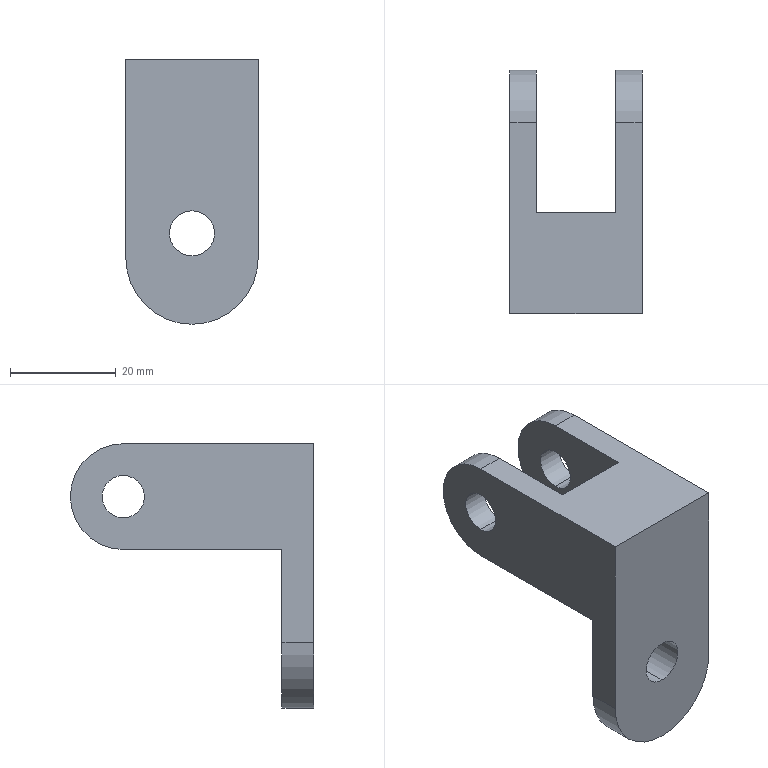Part | SolidWorks | features ICE 4, Fillet 2, Extrusion 1 | 1 solid | 19 faces | box 25 x 46 x 50 mm | volume 17741 mm3 | cylinder 10 | plane 9 | commonest cylinder face diameters 8 x4 8.5 x2 20 x2 25 x2
STEP:
#1=CARTESIAN_POINT('',(0.,0.,-12.065));
#2=VERTEX_POINT('',#1);
#3=CARTESIAN_POINT('',(0.,0.,-3.565));
#4=VERTEX_POINT('',#3);
#5=CARTESIAN_POINT('',(0.,0.,-7.815));
#6=DIRECTION('',(0.,1.,0.));
#7=DIRECTION('',(0.,0.,1.));
#8=AXIS2_PLACEMENT_3D('',#5,#6,#7);
#9=CIRCLE('',#8,4.25);
#10=EDGE_CURVE('',#2,#4,#9,.T.);
#11=ORIENTED_EDGE('',*,*,#10,.F.);
#12=CARTESIAN_POINT('',(0.,6.,-12.065));
#13=VERTEX_POINT('',#12);
#14=CARTESIAN_POINT('',(0.,0.,-12.065));
#15=DIRECTION('',(0.,1.,0.));
#16=VECTOR('',#15,1000.);
#17=LINE('',#14,#16);
#18=EDGE_CURVE('',#2,#13,#17,.T.);
#19=ORIENTED_EDGE('',*,*,#18,.T.);
#20=CARTESIAN_POINT('',(0.,6.,-3.565));
#21=VERTEX_POINT('',#20);
#22=CARTESIAN_POINT('',(0.,6.,-7.815));
#23=DIRECTION('',(0.,1.,0.));
#24=DIRECTION('',(0.,0.,1.));
#25=AXIS2_PLACEMENT_3D('',#22,#23,#24);
#26=CIRCLE('',#25,4.25);
#27=EDGE_CURVE('',#13,#21,#26,.T.);
#28=ORIENTED_EDGE('',*,*,#27,.T.);
#29=CARTESIAN_POINT('',(0.,0.,-3.565));
#30=DIRECTION('',(0.,1.,0.));
#31=VECTOR('',#30,1000.);
#32=LINE('',#29,#31);
#33=EDGE_CURVE('',#4,#21,#32,.T.);
#34=ORIENTED_EDGE('',*,*,#33,.F.);
#35=EDGE_LOOP('',(#11,#19,#28,#34));
#36=FACE_OUTER_BOUND('',#35,.T.);
#37=CARTESIAN_POINT('',(0.,0.,-7.815));
#38=DIRECTION('',(0.,1.,0.));
#39=DIRECTION('',(0.,0.,1.));
#40=AXIS2_PLACEMENT_3D('',#37,#38,#39);
#41=CYLINDRICAL_SURFACE('',#40,4.25);
#42=ADVANCED_FACE('',(#36),#41,.F.);
#43=CARTESIAN_POINT('',(12.5,36.,11.));
#44=VERTEX_POINT('',#43);
#45=CARTESIAN_POINT('',(12.5,36.,19.));
#46=VERTEX_POINT('',#45);
#47=CARTESIAN_POINT('',(12.5,36.,15.));
#48=DIRECTION('',(-1.,0.,0.));
#49=DIRECTION('',(0.,0.,1.));
#50=AXIS2_PLACEMENT_3D('',#47,#48,#49);
#51=CIRCLE('',#50,4.);
#52=EDGE_CURVE('',#44,#46,#51,.T.);
#53=ORIENTED_EDGE('',*,*,#52,.F.);
#54=CARTESIAN_POINT('',(7.5,36.,11.));
#55=VERTEX_POINT('',#54);
#56=CARTESIAN_POINT('',(12.5,36.,11.));
#57=DIRECTION('',(-1.,0.,0.));
#58=VECTOR('',#57,1000.);
#59=LINE('',#56,#58);
#60=EDGE_CURVE('',#44,#55,#59,.T.);
#61=ORIENTED_EDGE('',*,*,#60,.T.);
#62=CARTESIAN_POINT('',(7.5,36.,19.));
#63=VERTEX_POINT('',#62);
#64=CARTESIAN_POINT('',(7.5,36.,15.));
#65=DIRECTION('',(1.,0.,0.));
#66=DIRECTION('',(0.,0.,-1.));
#67=AXIS2_PLACEMENT_3D('',#64,#65,#66);
#68=CIRCLE('',#67,4.);
#69=EDGE_CURVE('',#63,#55,#68,.T.);
#70=ORIENTED_EDGE('',*,*,#69,.F.);
#71=CARTESIAN_POINT('',(12.5,36.,19.));
#72=DIRECTION('',(-1.,0.,0.));
#73=VECTOR('',#72,1000.);
#74=LINE('',#71,#73);
#75=EDGE_CURVE('',#46,#63,#74,.T.);
#76=ORIENTED_EDGE('',*,*,#75,.F.);
#77=EDGE_LOOP('',(#53,#61,#70,#76));
#78=FACE_OUTER_BOUND('',#77,.T.);
#79=CARTESIAN_POINT('',(12.5,36.,15.));
#80=DIRECTION('',(-1.,0.,0.));
#81=DIRECTION('',(0.,0.,1.));
#82=AXIS2_PLACEMENT_3D('',#79,#80,#81);
#83=CYLINDRICAL_SURFACE('',#82,4.);
#84=ADVANCED_FACE('',(#78),#83,.F.);
#85=CARTESIAN_POINT('',(-7.5,36.,19.));
#86=VERTEX_POINT('',#85);
#87=CARTESIAN_POINT('',(-7.5,36.,11.));
#88=VERTEX_POINT('',#87);
#89=CARTESIAN_POINT('',(-7.5,36.,15.));
#90=DIRECTION('',(1.,0.,0.));
#91=DIRECTION('',(0.,0.,-1.));
#92=AXIS2_PLACEMENT_3D('',#89,#90,#91);
#93=CIRCLE('',#92,4.);
#94=EDGE_CURVE('',#86,#88,#93,.T.);
#95=ORIENTED_EDGE('',*,*,#94,.T.);
#96=CARTESIAN_POINT('',(-12.5,36.,11.));
#97=VERTEX_POINT('',#96);
#98=CARTESIAN_POINT('',(12.5,36.,11.));
#99=DIRECTION('',(-1.,0.,0.));
#100=VECTOR('',#99,1000.);
#101=LINE('',#98,#100);
#102=EDGE_CURVE('',#88,#97,#101,.T.);
#103=ORIENTED_EDGE('',*,*,#102,.T.);
#104=CARTESIAN_POINT('',(-12.5,36.,19.));
#105=VERTEX_POINT('',#104);
#106=CARTESIAN_POINT('',(-12.5,36.,15.));
#107=DIRECTION('',(-1.,0.,0.));
#108=DIRECTION('',(0.,0.,1.));
#109=AXIS2_PLACEMENT_3D('',#106,#107,#108);
#110=CIRCLE('',#109,4.);
#111=EDGE_CURVE('',#97,#105,#110,.T.);
#112=ORIENTED_EDGE('',*,*,#111,.T.);
#113=CARTESIAN_POINT('',(12.5,36.,19.));
#114=DIRECTION('',(-1.,0.,0.));
#115=VECTOR('',#114,1000.);
#116=LINE('',#113,#115);
#117=EDGE_CURVE('',#86,#105,#116,.T.);
#118=ORIENTED_EDGE('',*,*,#117,.F.);
#119=EDGE_LOOP('',(#95,#103,#112,#118));
#120=FACE_OUTER_BOUND('',#119,.T.);
#121=CARTESIAN_POINT('',(12.5,36.,15.));
#122=DIRECTION('',(-1.,0.,0.));
#123=DIRECTION('',(0.,0.,1.));
#124=AXIS2_PLACEMENT_3D('',#121,#122,#123);
#125=CYLINDRICAL_SURFACE('',#124,4.);
#126=ADVANCED_FACE('',(#120),#125,.F.);
#127=CARTESIAN_POINT('',(0.,6.,-25.));
#128=VERTEX_POINT('',#127);
#129=CARTESIAN_POINT('',(-12.5,6.,-12.5));
#130=VERTEX_POINT('',#129);
#131=CARTESIAN_POINT('',(0.,6.,-12.5));
#132=DIRECTION('',(0.,1.,0.));
#133=DIRECTION('',(0.,0.,-1.));
#134=AXIS2_PLACEMENT_3D('',#131,#132,#133);
#135=CIRCLE('',#134,12.5);
#136=EDGE_CURVE('',#128,#130,#135,.T.);
#137=ORIENTED_EDGE('',*,*,#136,.F.);
#138=CARTESIAN_POINT('',(0.,0.,-25.));
#139=VERTEX_POINT('',#138);
#140=CARTESIAN_POINT('',(0.,6.,-25.));
#141=DIRECTION('',(0.,-1.,0.));
#142=VECTOR('',#141,1000.);
#143=LINE('',#140,#142);
#144=EDGE_CURVE('',#128,#139,#143,.T.);
#145=ORIENTED_EDGE('',*,*,#144,.T.);
#146=CARTESIAN_POINT('',(-12.5,0.,-12.5));
#147=VERTEX_POINT('',#146);
#148=CARTESIAN_POINT('',(0.,0.,-12.5));
#149=DIRECTION('',(0.,-1.,0.));
#150=DIRECTION('',(0.,0.,-1.));
#151=AXIS2_PLACEMENT_3D('',#148,#149,#150);
#152=CIRCLE('',#151,12.5);
#153=EDGE_CURVE('',#147,#139,#152,.T.);
#154=ORIENTED_EDGE('',*,*,#153,.F.);
#155=CARTESIAN_POINT('',(-12.5,6.,-12.5));
#156=DIRECTION('',(0.,-1.,0.));
#157=VECTOR('',#156,1000.);
#158=LINE('',#155,#157);
#159=EDGE_CURVE('',#130,#147,#158,.T.);
#160=ORIENTED_EDGE('',*,*,#159,.F.);
#161=EDGE_LOOP('',(#137,#145,#154,#160));
#162=FACE_OUTER_BOUND('',#161,.T.);
#163=CARTESIAN_POINT('',(0.,6.,-12.5));
#164=DIRECTION('',(0.,-1.,0.));
#165=DIRECTION('',(0.,0.,-1.));
#166=AXIS2_PLACEMENT_3D('',#163,#164,#165);
#167=CYLINDRICAL_SURFACE('',#166,12.5);
#168=ADVANCED_FACE('',(#162),#167,.T.);
#169=CARTESIAN_POINT('',(-7.5,36.,25.));
#170=VERTEX_POINT('',#169);
#171=CARTESIAN_POINT('',(-12.5,36.,25.));
#172=VERTEX_POINT('',#171);
#173=CARTESIAN_POINT('',(-12.5,36.,25.));
#174=DIRECTION('',(-1.,0.,0.));
#175=VECTOR('',#174,1000.);
#176=LINE('',#173,#175);
#177=EDGE_CURVE('',#170,#172,#176,.T.);
#178=ORIENTED_EDGE('',*,*,#177,.F.);
#179=CARTESIAN_POINT('',(-7.5,36.,5.));
#180=VERTEX_POINT('',#179);
#181=CARTESIAN_POINT('',(-7.5,36.,15.));
#182=DIRECTION('',(-1.,0.,0.));
#183=DIRECTION('',(0.,0.,-1.));
#184=AXIS2_PLACEMENT_3D('',#181,#182,#183);
#185=CIRCLE('',#184,10.);
#186=EDGE_CURVE('',#170,#180,#185,.T.);
#187=ORIENTED_EDGE('',*,*,#186,.T.);
#188=CARTESIAN_POINT('',(-12.5,36.,5.));
#189=VERTEX_POINT('',#188);
#190=CARTESIAN_POINT('',(-12.5,36.,5.));
#191=DIRECTION('',(1.,0.,0.));
#192=VECTOR('',#191,1000.);
#193=LINE('',#190,#192);
#194=EDGE_CURVE('',#189,#180,#193,.T.);
#195=ORIENTED_EDGE('',*,*,#194,.F.);
#196=CARTESIAN_POINT('',(-12.5,36.,15.));
#197=DIRECTION('',(-1.,0.,0.));
#198=DIRECTION('',(0.,0.,-1.));
#199=AXIS2_PLACEMENT_3D('',#196,#197,#198);
#200=CIRCLE('',#199,10.);
#201=EDGE_CURVE('',#172,#189,#200,.T.);
#202=ORIENTED_EDGE('',*,*,#201,.F.);
#203=EDGE_LOOP('',(#178,#187,#195,#202));
#204=FACE_OUTER_BOUND('',#203,.T.);
#205=CARTESIAN_POINT('',(-12.5,36.,15.));
#206=DIRECTION('',(-1.,0.,0.));
#207=DIRECTION('',(0.,0.,1.));
#208=AXIS2_PLACEMENT_3D('',#205,#206,#207);
#209=CYLINDRICAL_SURFACE('',#208,10.);
#210=ADVANCED_FACE('',(#204),#209,.T.);
#211=CARTESIAN_POINT('',(7.5,36.,25.));
#212=VERTEX_POINT('',#211);
#213=CARTESIAN_POINT('',(7.5,36.,5.));
#214=VERTEX_POINT('',#213);
#215=CARTESIAN_POINT('',(7.5,36.,15.));
#216=DIRECTION('',(-1.,0.,0.));
#217=DIRECTION('',(0.,0.,-1.));
#218=AXIS2_PLACEMENT_3D('',#215,#216,#217);
#219=CIRCLE('',#218,10.);
#220=EDGE_CURVE('',#212,#214,#219,.T.);
#221=ORIENTED_EDGE('',*,*,#220,.F.);
#222=CARTESIAN_POINT('',(12.5,36.,25.));
#223=VERTEX_POINT('',#222);
#224=CARTESIAN_POINT('',(-12.5,36.,25.));
#225=DIRECTION('',(-1.,0.,0.));
#226=VECTOR('',#225,1000.);
#227=LINE('',#224,#226);
#228=EDGE_CURVE('',#223,#212,#227,.T.);
#229=ORIENTED_EDGE('',*,*,#228,.F.);
#230=CARTESIAN_POINT('',(12.5,36.,5.));
#231=VERTEX_POINT('',#230);
#232=CARTESIAN_POINT('',(12.5,36.,15.));
#233=DIRECTION('',(1.,0.,0.));
#234=DIRECTION('',(0.,0.,1.));
#235=AXIS2_PLACEMENT_3D('',#232,#233,#234);
#236=CIRCLE('',#235,10.);
#237=EDGE_CURVE('',#231,#223,#236,.T.);
#238=ORIENTED_EDGE('',*,*,#237,.F.);
#239=CARTESIAN_POINT('',(-12.5,36.,5.));
#240=DIRECTION('',(1.,0.,0.));
#241=VECTOR('',#240,1000.);
#242=LINE('',#239,#241);
#243=EDGE_CURVE('',#214,#231,#242,.T.);
#244=ORIENTED_EDGE('',*,*,#243,.F.);
#245=EDGE_LOOP('',(#221,#229,#238,#244));
#246=FACE_OUTER_BOUND('',#245,.T.);
#247=CARTESIAN_POINT('',(-12.5,36.,15.));
#248=DIRECTION('',(-1.,0.,0.));
#249=DIRECTION('',(0.,0.,1.));
#250=AXIS2_PLACEMENT_3D('',#247,#248,#249);
#251=CYLINDRICAL_SURFACE('',#250,10.);
#252=ADVANCED_FACE('',(#246),#251,.T.);
#253=ORIENTED_EDGE('',*,*,#144,.F.);
#254=CARTESIAN_POINT('',(12.5,6.,-12.5));
#255=VERTEX_POINT('',#254);
#256=CARTESIAN_POINT('',(0.,6.,-12.5));
#257=DIRECTION('',(0.,1.,0.));
#258=DIRECTION('',(0.,0.,-1.));
#259=AXIS2_PLACEMENT_3D('',#256,#257,#258);
#260=CIRCLE('',#259,12.5);
#261=EDGE_CURVE('',#255,#128,#260,.T.);
#262=ORIENTED_EDGE('',*,*,#261,.F.);
#263=CARTESIAN_POINT('',(12.5,0.,-12.5));
#264=VERTEX_POINT('',#263);
#265=CARTESIAN_POINT('',(12.5,6.,-12.5));
#266=DIRECTION('',(0.,1.,0.));
#267=VECTOR('',#266,1000.);
#268=LINE('',#265,#267);
#269=EDGE_CURVE('',#264,#255,#268,.T.);
#270=ORIENTED_EDGE('',*,*,#269,.F.);
#271=CARTESIAN_POINT('',(0.,0.,-12.5));
#272=DIRECTION('',(0.,-1.,0.));
#273=DIRECTION('',(0.,0.,-1.));
#274=AXIS2_PLACEMENT_3D('',#271,#272,#273);
#275=CIRCLE('',#274,12.5);
#276=EDGE_CURVE('',#139,#264,#275,.T.);
#277=ORIENTED_EDGE('',*,*,#276,.F.);
#278=EDGE_LOOP('',(#253,#262,#270,#277));
#279=FACE_OUTER_BOUND('',#278,.T.);
#280=CARTESIAN_POINT('',(0.,6.,-12.5));
#281=DIRECTION('',(0.,-1.,0.));
#282=DIRECTION('',(0.,0.,-1.));
#283=AXIS2_PLACEMENT_3D('',#280,#281,#282);
#284=CYLINDRICAL_SURFACE('',#283,12.5);
#285=ADVANCED_FACE('',(#279),#284,.T.);
#286=CARTESIAN_POINT('',(0.,6.,-7.815));
#287=DIRECTION('',(0.,1.,0.));
#288=DIRECTION('',(0.,0.,1.));
#289=AXIS2_PLACEMENT_3D('',#286,#287,#288);
#290=CIRCLE('',#289,4.25);
#291=EDGE_CURVE('',#21,#13,#290,.T.);
#292=ORIENTED_EDGE('',*,*,#291,.F.);
#293=ORIENTED_EDGE('',*,*,#27,.F.);
#294=EDGE_LOOP('',(#292,#293));
#295=FACE_BOUND('',#294,.T.);
#296=CARTESIAN_POINT('',(12.5,6.,5.));
#297=VERTEX_POINT('',#296);
#298=CARTESIAN_POINT('',(12.5,6.,25.));
#299=DIRECTION('',(0.,0.,-1.));
#300=VECTOR('',#299,1000.);
#301=LINE('',#298,#300);
#302=EDGE_CURVE('',#297,#255,#301,.T.);
#303=ORIENTED_EDGE('',*,*,#302,.T.);
#304=ORIENTED_EDGE('',*,*,#261,.T.);
#305=ORIENTED_EDGE('',*,*,#136,.T.);
#306=CARTESIAN_POINT('',(-12.5,6.,5.));
#307=VERTEX_POINT('',#306);
#308=CARTESIAN_POINT('',(-12.5,6.,25.));
#309=DIRECTION('',(0.,0.,1.));
#310=VECTOR('',#309,1000.);
#311=LINE('',#308,#310);
#312=EDGE_CURVE('',#130,#307,#311,.T.);
#313=ORIENTED_EDGE('',*,*,#312,.T.);
#314=CARTESIAN_POINT('',(12.5,6.,5.));
#315=DIRECTION('',(-1.,0.,0.));
#316=VECTOR('',#315,1000.);
#317=LINE('',#314,#316);
#318=EDGE_CURVE('',#297,#307,#317,.T.);
#319=ORIENTED_EDGE('',*,*,#318,.F.);
#320=EDGE_LOOP('',(#303,#304,#305,#313,#319));
#321=FACE_OUTER_BOUND('',#320,.T.);
#322=CARTESIAN_POINT('',(0.,6.,0.));
#323=DIRECTION('',(0.,-1.,0.));
#324=DIRECTION('',(0.,0.,-1.));
#325=AXIS2_PLACEMENT_3D('',#322,#323,#324);
#326=PLANE('',#325);
#327=ADVANCED_FACE('',(#295,#321),#326,.F.);
#328=CARTESIAN_POINT('',(12.5,36.,15.));
#329=DIRECTION('',(-1.,0.,0.));
#330=DIRECTION('',(0.,0.,1.));
#331=AXIS2_PLACEMENT_3D('',#328,#329,#330);
#332=CIRCLE('',#331,4.);
#333=EDGE_CURVE('',#46,#44,#332,.T.);
#334=ORIENTED_EDGE('',*,*,#333,.T.);
#335=ORIENTED_EDGE('',*,*,#52,.T.);
#336=EDGE_LOOP('',(#334,#335));
#337=FACE_BOUND('',#336,.T.);
#338=CARTESIAN_POINT('',(12.5,46.,5.));
#339=DIRECTION('',(0.,-1.,0.));
#340=VECTOR('',#339,1000.);
#341=LINE('',#338,#340);
#342=EDGE_CURVE('',#231,#297,#341,.T.);
#343=ORIENTED_EDGE('',*,*,#342,.F.);
#344=ORIENTED_EDGE('',*,*,#237,.T.);
#345=CARTESIAN_POINT('',(12.5,0.,25.));
#346=VERTEX_POINT('',#345);
#347=CARTESIAN_POINT('',(12.5,6.,25.));
#348=DIRECTION('',(0.,-1.,0.));
#349=VECTOR('',#348,1000.);
#350=LINE('',#347,#349);
#351=EDGE_CURVE('',#223,#346,#350,.T.);
#352=ORIENTED_EDGE('',*,*,#351,.T.);
#353=CARTESIAN_POINT('',(12.5,0.,25.));
#354=DIRECTION('',(0.,0.,-1.));
#355=VECTOR('',#354,1000.);
#356=LINE('',#353,#355);
#357=EDGE_CURVE('',#346,#264,#356,.T.);
#358=ORIENTED_EDGE('',*,*,#357,.T.);
#359=ORIENTED_EDGE('',*,*,#269,.T.);
#360=ORIENTED_EDGE('',*,*,#302,.F.);
#361=EDGE_LOOP('',(#343,#344,#352,#358,#359,#360));
#362=FACE_OUTER_BOUND('',#361,.T.);
#363=CARTESIAN_POINT('',(12.5,6.,25.));
#364=DIRECTION('',(-1.,0.,0.));
#365=DIRECTION('',(0.,0.,1.));
#366=AXIS2_PLACEMENT_3D('',#363,#364,#365);
#367=PLANE('',#366);
#368=ADVANCED_FACE('',(#337,#362),#367,.F.);
#369=CARTESIAN_POINT('',(-12.5,36.,15.));
#370=DIRECTION('',(-1.,0.,0.));
#371=DIRECTION('',(0.,0.,1.));
#372=AXIS2_PLACEMENT_3D('',#369,#370,#371);
#373=CIRCLE('',#372,4.);
#374=EDGE_CURVE('',#105,#97,#373,.T.);
#375=ORIENTED_EDGE('',*,*,#374,.F.);
#376=ORIENTED_EDGE('',*,*,#111,.F.);
#377=EDGE_LOOP('',(#375,#376));
#378=FACE_BOUND('',#377,.T.);
#379=CARTESIAN_POINT('',(-12.5,0.,25.));
#380=VERTEX_POINT('',#379);
#381=CARTESIAN_POINT('',(-12.5,6.,25.));
#382=DIRECTION('',(0.,-1.,0.));
#383=VECTOR('',#382,1000.);
#384=LINE('',#381,#383);
#385=EDGE_CURVE('',#172,#380,#384,.T.);
#386=ORIENTED_EDGE('',*,*,#385,.F.);
#387=ORIENTED_EDGE('',*,*,#201,.T.);
#388=CARTESIAN_POINT('',(-12.5,46.,5.));
#389=DIRECTION('',(0.,-1.,0.));
#390=VECTOR('',#389,1000.);
#391=LINE('',#388,#390);
#392=EDGE_CURVE('',#189,#307,#391,.T.);
#393=ORIENTED_EDGE('',*,*,#392,.T.);
#394=ORIENTED_EDGE('',*,*,#312,.F.);
#395=ORIENTED_EDGE('',*,*,#159,.T.);
#396=CARTESIAN_POINT('',(-12.5,0.,25.));
#397=DIRECTION('',(0.,0.,1.));
#398=VECTOR('',#397,1000.);
#399=LINE('',#396,#398);
#400=EDGE_CURVE('',#147,#380,#399,.T.);
#401=ORIENTED_EDGE('',*,*,#400,.T.);
#402=EDGE_LOOP('',(#386,#387,#393,#394,#395,#401));
#403=FACE_OUTER_BOUND('',#402,.T.);
#404=CARTESIAN_POINT('',(-12.5,6.,25.));
#405=DIRECTION('',(1.,0.,0.));
#406=DIRECTION('',(0.,0.,-1.));
#407=AXIS2_PLACEMENT_3D('',#404,#405,#406);
#408=PLANE('',#407);
#409=ADVANCED_FACE('',(#378,#403),#408,.F.);
#410=ORIENTED_EDGE('',*,*,#228,.T.);
#411=CARTESIAN_POINT('',(7.5,19.053,25.));
#412=VERTEX_POINT('',#411);
#413=CARTESIAN_POINT('',(7.5,6.,25.));
#414=DIRECTION('',(0.,-1.,0.));
#415=VECTOR('',#414,1000.);
#416=LINE('',#413,#415);
#417=EDGE_CURVE('',#212,#412,#416,.T.);
#418=ORIENTED_EDGE('',*,*,#417,.T.);
#419=CARTESIAN_POINT('',(-7.5,19.053,25.));
#420=VERTEX_POINT('',#419);
#421=CARTESIAN_POINT('',(-12.5,19.053,25.));
#422=DIRECTION('',(-1.,0.,0.));
#423=VECTOR('',#422,1000.);
#424=LINE('',#421,#423);
#425=EDGE_CURVE('',#412,#420,#424,.T.);
#426=ORIENTED_EDGE('',*,*,#425,.T.);
#427=CARTESIAN_POINT('',(-7.5,6.,25.));
#428=DIRECTION('',(0.,-1.,0.));
#429=VECTOR('',#428,1000.);
#430=LINE('',#427,#429);
#431=EDGE_CURVE('',#170,#420,#430,.T.);
#432=ORIENTED_EDGE('',*,*,#431,.F.);
#433=ORIENTED_EDGE('',*,*,#177,.T.);
#434=ORIENTED_EDGE('',*,*,#385,.T.);
#435=CARTESIAN_POINT('',(-12.5,0.,25.));
#436=DIRECTION('',(1.,0.,0.));
#437=VECTOR('',#436,1000.);
#438=LINE('',#435,#437);
#439=EDGE_CURVE('',#380,#346,#438,.T.);
#440=ORIENTED_EDGE('',*,*,#439,.T.);
#441=ORIENTED_EDGE('',*,*,#351,.F.);
#442=EDGE_LOOP('',(#410,#418,#426,#432,#433,#434,#440,#441));
#443=FACE_OUTER_BOUND('',#442,.T.);
#444=CARTESIAN_POINT('',(-12.5,6.,25.));
#445=DIRECTION('',(0.,0.,-1.));
#446=DIRECTION('',(-1.,0.,0.));
#447=AXIS2_PLACEMENT_3D('',#444,#445,#446);
#448=PLANE('',#447);
#449=ADVANCED_FACE('',(#443),#448,.F.);
#450=CARTESIAN_POINT('',(0.,0.,-7.815));
#451=DIRECTION('',(0.,1.,0.));
#452=DIRECTION('',(0.,0.,1.));
#453=AXIS2_PLACEMENT_3D('',#450,#451,#452);
#454=CIRCLE('',#453,4.25);
#455=EDGE_CURVE('',#4,#2,#454,.T.);
#456=ORIENTED_EDGE('',*,*,#455,.T.);
#457=ORIENTED_EDGE('',*,*,#10,.T.);
#458=EDGE_LOOP('',(#456,#457));
#459=FACE_BOUND('',#458,.T.);
#460=ORIENTED_EDGE('',*,*,#400,.F.);
#461=ORIENTED_EDGE('',*,*,#153,.T.);
#462=ORIENTED_EDGE('',*,*,#276,.T.);
#463=ORIENTED_EDGE('',*,*,#357,.F.);
#464=ORIENTED_EDGE('',*,*,#439,.F.);
#465=EDGE_LOOP('',(#460,#461,#462,#463,#464));
#466=FACE_OUTER_BOUND('',#465,.T.);
#467=CARTESIAN_POINT('',(0.,0.,0.));
#468=DIRECTION('',(0.,-1.,0.));
#469=DIRECTION('',(0.,0.,-1.));
#470=AXIS2_PLACEMENT_3D('',#467,#468,#469);
#471=PLANE('',#470);
#472=ADVANCED_FACE('',(#459,#466),#471,.T.);
#473=CARTESIAN_POINT('',(7.5,19.053,5.));
#474=VERTEX_POINT('',#473);
#475=CARTESIAN_POINT('',(-7.5,19.053,5.));
#476=VERTEX_POINT('',#475);
#477=CARTESIAN_POINT('',(7.5,19.053,5.));
#478=DIRECTION('',(-1.,0.,0.));
#479=VECTOR('',#478,1000.);
#480=LINE('',#477,#479);
#481=EDGE_CURVE('',#474,#476,#480,.T.);
#482=ORIENTED_EDGE('',*,*,#481,.F.);
#483=CARTESIAN_POINT('',(7.5,46.,5.));
#484=DIRECTION('',(0.,1.,0.));
#485=VECTOR('',#484,1000.);
#486=LINE('',#483,#485);
#487=EDGE_CURVE('',#474,#214,#486,.T.);
#488=ORIENTED_EDGE('',*,*,#487,.T.);
#489=ORIENTED_EDGE('',*,*,#243,.T.);
#490=ORIENTED_EDGE('',*,*,#342,.T.);
#491=ORIENTED_EDGE('',*,*,#318,.T.);
#492=ORIENTED_EDGE('',*,*,#392,.F.);
#493=ORIENTED_EDGE('',*,*,#194,.T.);
#494=CARTESIAN_POINT('',(-7.5,46.,5.));
#495=DIRECTION('',(0.,1.,0.));
#496=VECTOR('',#495,1000.);
#497=LINE('',#494,#496);
#498=EDGE_CURVE('',#476,#180,#497,.T.);
#499=ORIENTED_EDGE('',*,*,#498,.F.);
#500=EDGE_LOOP('',(#482,#488,#489,#490,#491,#492,#493,#499));
#501=FACE_OUTER_BOUND('',#500,.T.);
#502=CARTESIAN_POINT('',(12.5,46.,5.));
#503=DIRECTION('',(0.,0.,1.));
#504=DIRECTION('',(1.,0.,0.));
#505=AXIS2_PLACEMENT_3D('',#502,#503,#504);
#506=PLANE('',#505);
#507=ADVANCED_FACE('',(#501),#506,.F.);
#508=CARTESIAN_POINT('',(7.5,19.053,5.));
#509=DIRECTION('',(0.,0.,1.));
#510=VECTOR('',#509,1000.);
#511=LINE('',#508,#510);
#512=EDGE_CURVE('',#474,#412,#511,.T.);
#513=ORIENTED_EDGE('',*,*,#512,.F.);
#514=ORIENTED_EDGE('',*,*,#481,.T.);
#515=CARTESIAN_POINT('',(-7.5,19.053,5.));
#516=DIRECTION('',(0.,0.,1.));
#517=VECTOR('',#516,1000.);
#518=LINE('',#515,#517);
#519=EDGE_CURVE('',#476,#420,#518,.T.);
#520=ORIENTED_EDGE('',*,*,#519,.T.);
#521=ORIENTED_EDGE('',*,*,#425,.F.);
#522=EDGE_LOOP('',(#513,#514,#520,#521));
#523=FACE_OUTER_BOUND('',#522,.T.);
#524=CARTESIAN_POINT('',(7.5,19.053,5.));
#525=DIRECTION('',(0.,-1.,0.));
#526=DIRECTION('',(0.,0.,-1.));
#527=AXIS2_PLACEMENT_3D('',#524,#525,#526);
#528=PLANE('',#527);
#529=ADVANCED_FACE('',(#523),#528,.F.);
#530=ORIENTED_EDGE('',*,*,#69,.T.);
#531=CARTESIAN_POINT('',(7.5,36.,15.));
#532=DIRECTION('',(1.,0.,0.));
#533=DIRECTION('',(0.,0.,-1.));
#534=AXIS2_PLACEMENT_3D('',#531,#532,#533);
#535=CIRCLE('',#534,4.);
#536=EDGE_CURVE('',#55,#63,#535,.T.);
#537=ORIENTED_EDGE('',*,*,#536,.T.);
#538=EDGE_LOOP('',(#530,#537));
#539=FACE_BOUND('',#538,.T.);
#540=ORIENTED_EDGE('',*,*,#220,.T.);
#541=ORIENTED_EDGE('',*,*,#487,.F.);
#542=ORIENTED_EDGE('',*,*,#512,.T.);
#543=ORIENTED_EDGE('',*,*,#417,.F.);
#544=EDGE_LOOP('',(#540,#541,#542,#543));
#545=FACE_OUTER_BOUND('',#544,.T.);
#546=CARTESIAN_POINT('',(7.5,0.,0.));
#547=DIRECTION('',(1.,0.,0.));
#548=DIRECTION('',(0.,0.,-1.));
#549=AXIS2_PLACEMENT_3D('',#546,#547,#548);
#550=PLANE('',#549);
#551=ADVANCED_FACE('',(#539,#545),#550,.F.);
#552=ORIENTED_EDGE('',*,*,#94,.F.);
#553=CARTESIAN_POINT('',(-7.5,36.,15.));
#554=DIRECTION('',(1.,0.,0.));
#555=DIRECTION('',(0.,0.,-1.));
#556=AXIS2_PLACEMENT_3D('',#553,#554,#555);
#557=CIRCLE('',#556,4.);
#558=EDGE_CURVE('',#88,#86,#557,.T.);
#559=ORIENTED_EDGE('',*,*,#558,.F.);
#560=EDGE_LOOP('',(#552,#559));
#561=FACE_BOUND('',#560,.T.);
#562=ORIENTED_EDGE('',*,*,#431,.T.);
#563=ORIENTED_EDGE('',*,*,#519,.F.);
#564=ORIENTED_EDGE('',*,*,#498,.T.);
#565=ORIENTED_EDGE('',*,*,#186,.F.);
#566=EDGE_LOOP('',(#562,#563,#564,#565));
#567=FACE_OUTER_BOUND('',#566,.T.);
#568=CARTESIAN_POINT('',(-7.5,0.,0.));
#569=DIRECTION('',(1.,0.,0.));
#570=DIRECTION('',(0.,0.,-1.));
#571=AXIS2_PLACEMENT_3D('',#568,#569,#570);
#572=PLANE('',#571);
#573=ADVANCED_FACE('',(#561,#567),#572,.T.);
#574=ORIENTED_EDGE('',*,*,#102,.F.);
#575=ORIENTED_EDGE('',*,*,#558,.T.);
#576=ORIENTED_EDGE('',*,*,#117,.T.);
#577=ORIENTED_EDGE('',*,*,#374,.T.);
#578=EDGE_LOOP('',(#574,#575,#576,#577));
#579=FACE_OUTER_BOUND('',#578,.T.);
#580=CARTESIAN_POINT('',(12.5,36.,15.));
#581=DIRECTION('',(-1.,0.,0.));
#582=DIRECTION('',(0.,0.,1.));
#583=AXIS2_PLACEMENT_3D('',#580,#581,#582);
#584=CYLINDRICAL_SURFACE('',#583,4.);
#585=ADVANCED_FACE('',(#579),#584,.F.);
#586=ORIENTED_EDGE('',*,*,#60,.F.);
#587=ORIENTED_EDGE('',*,*,#333,.F.);
#588=ORIENTED_EDGE('',*,*,#75,.T.);
#589=ORIENTED_EDGE('',*,*,#536,.F.);
#590=EDGE_LOOP('',(#586,#587,#588,#589));
#591=FACE_OUTER_BOUND('',#590,.T.);
#592=CARTESIAN_POINT('',(12.5,36.,15.));
#593=DIRECTION('',(-1.,0.,0.));
#594=DIRECTION('',(0.,0.,1.));
#595=AXIS2_PLACEMENT_3D('',#592,#593,#594);
#596=CYLINDRICAL_SURFACE('',#595,4.);
#597=ADVANCED_FACE('',(#591),#596,.F.);
#598=ORIENTED_EDGE('',*,*,#18,.F.);
#599=ORIENTED_EDGE('',*,*,#455,.F.);
#600=ORIENTED_EDGE('',*,*,#33,.T.);
#601=ORIENTED_EDGE('',*,*,#291,.T.);
#602=EDGE_LOOP('',(#598,#599,#600,#601));
#603=FACE_OUTER_BOUND('',#602,.T.);
#604=CARTESIAN_POINT('',(0.,0.,-7.815));
#605=DIRECTION('',(0.,1.,0.));
#606=DIRECTION('',(0.,0.,1.));
#607=AXIS2_PLACEMENT_3D('',#604,#605,#606);
#608=CYLINDRICAL_SURFACE('',#607,4.25);
#609=ADVANCED_FACE('',(#603),#608,.F.);
#610=CLOSED_SHELL('',(#42,#84,#126,#168,#210,#252,#285,#327,#368,#409,#449,#472,#507,#529,#551,#573,#585,#597,#609));
#611=MANIFOLD_SOLID_BREP('',#610);
#612=CARTESIAN_POINT('',(0.,0.,0.));
#613=DIRECTION('',(0.,0.,1.));
#614=DIRECTION('',(1.,0.,0.));
#615=AXIS2_PLACEMENT_3D('',#612,#613,#614);
#616=(LENGTH_UNIT()NAMED_UNIT(*)SI_UNIT(.MILLI.,.METRE.));
#617=UNCERTAINTY_MEASURE_WITH_UNIT(LENGTH_MEASURE(0.00001),#616,'','');
#618=(NAMED_UNIT(*)PLANE_ANGLE_UNIT()SI_UNIT($,.RADIAN.));
#619=(NAMED_UNIT(*)SI_UNIT($,.STERADIAN.)SOLID_ANGLE_UNIT());
#620=(GEOMETRIC_REPRESENTATION_CONTEXT(3)GLOBAL_UNCERTAINTY_ASSIGNED_CONTEXT((#617))GLOBAL_UNIT_ASSIGNED_CONTEXT((#616,#618,#619))REPRESENTATION_CONTEXT('',''));
#621=ADVANCED_BREP_SHAPE_REPRESENTATION('',(#611,#615),#620);